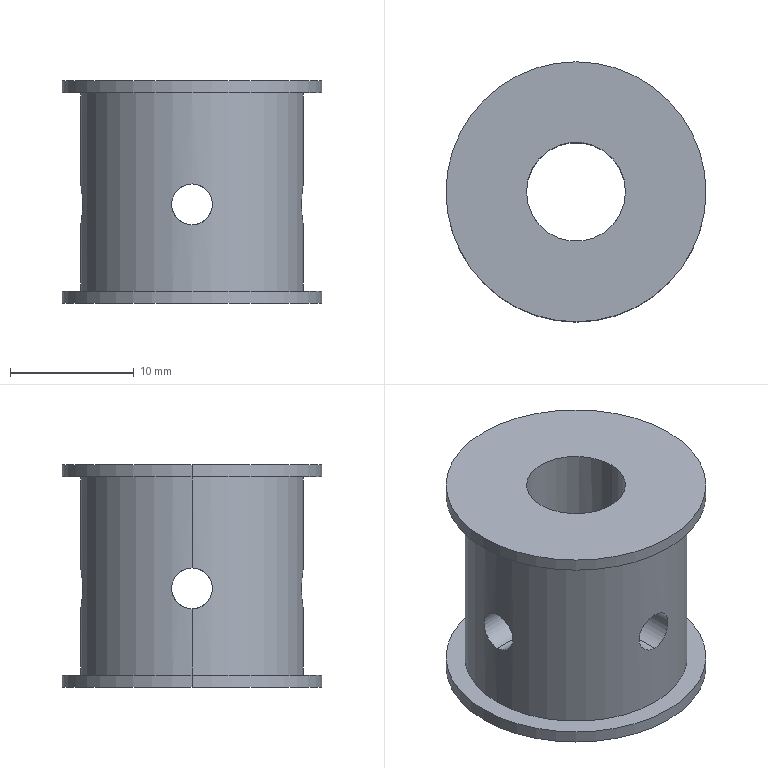Part | STEP file | 11-FG-SZ02211 | 1 solid | 20 faces | box 21 x 21 x 18 mm | volume 3687 mm3 | cylinder 16 | plane 4 | commonest cylinder face diameters 3.3 x8 21 x4 8 x2 18 x2
STEP:
#1=CARTESIAN_POINT('',(0.,-4.,9.65));
#2=VERTEX_POINT('',#1);
#3=CARTESIAN_POINT('',(0.,-4.,6.35));
#4=VERTEX_POINT('',#3);
#5=CARTESIAN_POINT('',(0.,-4.,9.65));
#6=CARTESIAN_POINT('',(0.1103,-4.,9.65));
#7=CARTESIAN_POINT('',(0.2186,-3.995,9.639));
#8=CARTESIAN_POINT('',(0.4313,-3.978,9.596));
#9=CARTESIAN_POINT('',(0.5367,-3.965,9.564));
#10=CARTESIAN_POINT('',(0.8358,-3.917,9.439));
#11=CARTESIAN_POINT('',(1.017,-3.872,9.316));
#12=CARTESIAN_POINT('',(1.318,-3.78,9.015));
#13=CARTESIAN_POINT('',(1.44,-3.733,8.834));
#14=CARTESIAN_POINT('',(1.564,-3.682,8.537));
#15=CARTESIAN_POINT('',(1.596,-3.668,8.432));
#16=CARTESIAN_POINT('',(1.639,-3.649,8.218));
#17=CARTESIAN_POINT('',(1.65,-3.644,8.11));
#18=CARTESIAN_POINT('',(1.65,-3.644,7.892));
#19=CARTESIAN_POINT('',(1.639,-3.649,7.781));
#20=CARTESIAN_POINT('',(1.596,-3.668,7.569));
#21=CARTESIAN_POINT('',(1.565,-3.682,7.465));
#22=CARTESIAN_POINT('',(1.481,-3.716,7.264));
#23=CARTESIAN_POINT('',(1.43,-3.736,7.17));
#24=CARTESIAN_POINT('',(1.311,-3.78,6.992));
#25=CARTESIAN_POINT('',(1.242,-3.803,6.908));
#26=CARTESIAN_POINT('',(1.091,-3.849,6.757));
#27=CARTESIAN_POINT('',(1.009,-3.872,6.69));
#28=CARTESIAN_POINT('',(0.8304,-3.914,6.57));
#29=CARTESIAN_POINT('',(0.7343,-3.933,6.519));
#30=CARTESIAN_POINT('',(0.4369,-3.981,6.394));
#31=CARTESIAN_POINT('',(0.2174,-4.,6.35));
#32=CARTESIAN_POINT('',(0.,-4.,6.35));
#33=B_SPLINE_CURVE_WITH_KNOTS('',3,(#5,#6,#7,#8,#9,#10,#11,#12,#13,#14,#15,#16,#17,#18,#19,#20,#21,#22,#23,#24,#25,#26,#27,#28,#29,#30,#31,#32),.UNSPECIFIED.,.F.,.F.,(4,2,2,2,2,2,2,2,2,2,2,2,2,4),(0.,0.0003261,0.0006522,0.001304,0.001957,0.002283,0.002609,0.002935,0.003261,0.003587,0.003913,0.004239,0.004565,0.005218),.UNSPECIFIED.);
#34=EDGE_CURVE('',#2,#4,#33,.T.);
#35=ORIENTED_EDGE('',*,*,#34,.F.);
#36=CARTESIAN_POINT('',(0.,-4.,6.35));
#37=CARTESIAN_POINT('',(-0.1086,-4.,6.35));
#38=CARTESIAN_POINT('',(-0.2188,-3.995,6.361));
#39=CARTESIAN_POINT('',(-0.4326,-3.978,6.404));
#40=CARTESIAN_POINT('',(-0.5359,-3.965,6.436));
#41=CARTESIAN_POINT('',(-0.8355,-3.917,6.561));
#42=CARTESIAN_POINT('',(-1.016,-3.872,6.682));
#43=CARTESIAN_POINT('',(-1.244,-3.803,6.91));
#44=CARTESIAN_POINT('',(-1.311,-3.78,6.992));
#45=CARTESIAN_POINT('',(-1.43,-3.736,7.17));
#46=CARTESIAN_POINT('',(-1.481,-3.716,7.266));
#47=CARTESIAN_POINT('',(-1.564,-3.682,7.465));
#48=CARTESIAN_POINT('',(-1.596,-3.668,7.567));
#49=CARTESIAN_POINT('',(-1.639,-3.649,7.78));
#50=CARTESIAN_POINT('',(-1.65,-3.644,7.891));
#51=CARTESIAN_POINT('',(-1.65,-3.644,8.217));
#52=CARTESIAN_POINT('',(-1.606,-3.665,8.436));
#53=CARTESIAN_POINT('',(-1.482,-3.716,8.734));
#54=CARTESIAN_POINT('',(-1.43,-3.736,8.83));
#55=CARTESIAN_POINT('',(-1.311,-3.78,9.008));
#56=CARTESIAN_POINT('',(-1.243,-3.803,9.09));
#57=CARTESIAN_POINT('',(-1.092,-3.849,9.242));
#58=CARTESIAN_POINT('',(-1.008,-3.872,9.311));
#59=CARTESIAN_POINT('',(-0.8311,-3.914,9.429));
#60=CARTESIAN_POINT('',(-0.7368,-3.933,9.48));
#61=CARTESIAN_POINT('',(-0.4348,-3.982,9.607));
#62=CARTESIAN_POINT('',(-0.2205,-4.,9.65));
#63=CARTESIAN_POINT('',(0.,-4.,9.65));
#64=B_SPLINE_CURVE_WITH_KNOTS('',3,(#36,#37,#38,#39,#40,#41,#42,#43,#44,#45,#46,#47,#48,#49,#50,#51,#52,#53,#54,#55,#56,#57,#58,#59,#60,#61,#62,#63),.UNSPECIFIED.,.F.,.F.,(4,2,2,2,2,2,2,2,2,2,2,2,2,4),(0.005218,0.005543,0.005869,0.006521,0.006847,0.007173,0.007499,0.007824,0.008476,0.008802,0.009128,0.009454,0.009779,0.01043),.UNSPECIFIED.);
#65=EDGE_CURVE('',#4,#2,#64,.T.);
#66=ORIENTED_EDGE('',*,*,#65,.F.);
#67=EDGE_LOOP('',(#35,#66));
#68=FACE_BOUND('',#67,.T.);
#69=CARTESIAN_POINT('',(4.,0.,18.));
#70=VERTEX_POINT('',#69);
#71=CARTESIAN_POINT('',(-4.,0.,18.));
#72=VERTEX_POINT('',#71);
#73=CARTESIAN_POINT('',(0.,0.,18.));
#74=DIRECTION('',(0.,0.,-1.));
#75=DIRECTION('',(-1.,0.,0.));
#76=AXIS2_PLACEMENT_3D('',#73,#74,#75);
#77=CIRCLE('',#76,4.);
#78=EDGE_CURVE('',#70,#72,#77,.T.);
#79=ORIENTED_EDGE('',*,*,#78,.F.);
#80=CARTESIAN_POINT('',(4.,0.,9.65));
#81=VERTEX_POINT('',#80);
#82=CARTESIAN_POINT('',(4.,0.,18.));
#83=DIRECTION('',(0.,0.,-1.));
#84=VECTOR('',#83,1000.);
#85=LINE('',#82,#84);
#86=EDGE_CURVE('',#70,#81,#85,.T.);
#87=ORIENTED_EDGE('',*,*,#86,.T.);
#88=CARTESIAN_POINT('',(4.,0.,6.35));
#89=VERTEX_POINT('',#88);
#90=CARTESIAN_POINT('',(4.,0.,6.35));
#91=CARTESIAN_POINT('',(4.,-0.1103,6.35));
#92=CARTESIAN_POINT('',(3.995,-0.2186,6.361));
#93=CARTESIAN_POINT('',(3.978,-0.4313,6.404));
#94=CARTESIAN_POINT('',(3.965,-0.5367,6.436));
#95=CARTESIAN_POINT('',(3.917,-0.8358,6.561));
#96=CARTESIAN_POINT('',(3.872,-1.017,6.684));
#97=CARTESIAN_POINT('',(3.78,-1.318,6.985));
#98=CARTESIAN_POINT('',(3.733,-1.44,7.166));
#99=CARTESIAN_POINT('',(3.682,-1.564,7.463));
#100=CARTESIAN_POINT('',(3.668,-1.596,7.568));
#101=CARTESIAN_POINT('',(3.649,-1.639,7.782));
#102=CARTESIAN_POINT('',(3.644,-1.65,7.89));
#103=CARTESIAN_POINT('',(3.644,-1.65,8.108));
#104=CARTESIAN_POINT('',(3.649,-1.639,8.219));
#105=CARTESIAN_POINT('',(3.668,-1.596,8.431));
#106=CARTESIAN_POINT('',(3.682,-1.565,8.535));
#107=CARTESIAN_POINT('',(3.716,-1.481,8.736));
#108=CARTESIAN_POINT('',(3.736,-1.43,8.83));
#109=CARTESIAN_POINT('',(3.78,-1.311,9.008));
#110=CARTESIAN_POINT('',(3.803,-1.242,9.092));
#111=CARTESIAN_POINT('',(3.849,-1.091,9.243));
#112=CARTESIAN_POINT('',(3.872,-1.009,9.31));
#113=CARTESIAN_POINT('',(3.914,-0.8304,9.43));
#114=CARTESIAN_POINT('',(3.933,-0.7343,9.481));
#115=CARTESIAN_POINT('',(3.981,-0.4369,9.606));
#116=CARTESIAN_POINT('',(4.,-0.2174,9.65));
#117=CARTESIAN_POINT('',(4.,0.,9.65));
#118=B_SPLINE_CURVE_WITH_KNOTS('',3,(#90,#91,#92,#93,#94,#95,#96,#97,#98,#99,#100,#101,#102,#103,#104,#105,#106,#107,#108,#109,#110,#111,#112,#113,#114,#115,#116,#117),.UNSPECIFIED.,.F.,.F.,(4,2,2,2,2,2,2,2,2,2,2,2,2,4),(0.,0.0003261,0.0006522,0.001304,0.001957,0.002283,0.002609,0.002935,0.003261,0.003587,0.003913,0.004239,0.004565,0.005218),.UNSPECIFIED.);
#119=EDGE_CURVE('',#89,#81,#118,.T.);
#120=ORIENTED_EDGE('',*,*,#119,.F.);
#121=CARTESIAN_POINT('',(4.,0.,0.));
#122=VERTEX_POINT('',#121);
#123=CARTESIAN_POINT('',(4.,0.,18.));
#124=DIRECTION('',(0.,0.,-1.));
#125=VECTOR('',#124,1000.);
#126=LINE('',#123,#125);
#127=EDGE_CURVE('',#89,#122,#126,.T.);
#128=ORIENTED_EDGE('',*,*,#127,.T.);
#129=CARTESIAN_POINT('',(-4.,0.,0.));
#130=VERTEX_POINT('',#129);
#131=CARTESIAN_POINT('',(0.,0.,0.));
#132=DIRECTION('',(0.,0.,-1.));
#133=DIRECTION('',(-1.,0.,0.));
#134=AXIS2_PLACEMENT_3D('',#131,#132,#133);
#135=CIRCLE('',#134,4.);
#136=EDGE_CURVE('',#122,#130,#135,.T.);
#137=ORIENTED_EDGE('',*,*,#136,.T.);
#138=CARTESIAN_POINT('',(-4.,0.,6.35));
#139=VERTEX_POINT('',#138);
#140=CARTESIAN_POINT('',(-4.,0.,18.));
#141=DIRECTION('',(0.,0.,-1.));
#142=VECTOR('',#141,1000.);
#143=LINE('',#140,#142);
#144=EDGE_CURVE('',#139,#130,#143,.T.);
#145=ORIENTED_EDGE('',*,*,#144,.F.);
#146=CARTESIAN_POINT('',(-4.,0.,9.65));
#147=VERTEX_POINT('',#146);
#148=CARTESIAN_POINT('',(-4.,0.,9.65));
#149=CARTESIAN_POINT('',(-4.,-0.1086,9.65));
#150=CARTESIAN_POINT('',(-3.995,-0.2188,9.639));
#151=CARTESIAN_POINT('',(-3.978,-0.4326,9.596));
#152=CARTESIAN_POINT('',(-3.965,-0.5359,9.564));
#153=CARTESIAN_POINT('',(-3.917,-0.8355,9.439));
#154=CARTESIAN_POINT('',(-3.872,-1.016,9.318));
#155=CARTESIAN_POINT('',(-3.803,-1.244,9.09));
#156=CARTESIAN_POINT('',(-3.78,-1.311,9.008));
#157=CARTESIAN_POINT('',(-3.736,-1.43,8.83));
#158=CARTESIAN_POINT('',(-3.716,-1.481,8.734));
#159=CARTESIAN_POINT('',(-3.682,-1.564,8.535));
#160=CARTESIAN_POINT('',(-3.668,-1.596,8.433));
#161=CARTESIAN_POINT('',(-3.649,-1.639,8.22));
#162=CARTESIAN_POINT('',(-3.644,-1.65,8.109));
#163=CARTESIAN_POINT('',(-3.644,-1.65,7.783));
#164=CARTESIAN_POINT('',(-3.665,-1.606,7.564));
#165=CARTESIAN_POINT('',(-3.716,-1.482,7.266));
#166=CARTESIAN_POINT('',(-3.736,-1.43,7.17));
#167=CARTESIAN_POINT('',(-3.78,-1.311,6.992));
#168=CARTESIAN_POINT('',(-3.803,-1.243,6.91));
#169=CARTESIAN_POINT('',(-3.849,-1.092,6.758));
#170=CARTESIAN_POINT('',(-3.872,-1.008,6.689));
#171=CARTESIAN_POINT('',(-3.914,-0.8311,6.571));
#172=CARTESIAN_POINT('',(-3.933,-0.7368,6.52));
#173=CARTESIAN_POINT('',(-3.982,-0.4348,6.393));
#174=CARTESIAN_POINT('',(-4.,-0.2205,6.35));
#175=CARTESIAN_POINT('',(-4.,0.,6.35));
#176=B_SPLINE_CURVE_WITH_KNOTS('',3,(#148,#149,#150,#151,#152,#153,#154,#155,#156,#157,#158,#159,#160,#161,#162,#163,#164,#165,#166,#167,#168,#169,#170,#171,#172,#173,#174,#175),.UNSPECIFIED.,.F.,.F.,(4,2,2,2,2,2,2,2,2,2,2,2,2,4),(0.005218,0.005543,0.005869,0.006521,0.006847,0.007173,0.007499,0.007824,0.008476,0.008802,0.009128,0.009454,0.009779,0.01043),.UNSPECIFIED.);
#177=EDGE_CURVE('',#147,#139,#176,.T.);
#178=ORIENTED_EDGE('',*,*,#177,.F.);
#179=CARTESIAN_POINT('',(-4.,0.,18.));
#180=DIRECTION('',(0.,0.,-1.));
#181=VECTOR('',#180,1000.);
#182=LINE('',#179,#181);
#183=EDGE_CURVE('',#72,#147,#182,.T.);
#184=ORIENTED_EDGE('',*,*,#183,.F.);
#185=EDGE_LOOP('',(#79,#87,#120,#128,#137,#145,#178,#184));
#186=FACE_OUTER_BOUND('',#185,.T.);
#187=CARTESIAN_POINT('',(0.,0.,18.));
#188=DIRECTION('',(0.,0.,-1.));
#189=DIRECTION('',(-1.,0.,0.));
#190=AXIS2_PLACEMENT_3D('',#187,#188,#189);
#191=CYLINDRICAL_SURFACE('',#190,4.);
#192=ADVANCED_FACE('',(#68,#186),#191,.F.);
#193=CARTESIAN_POINT('',(-9.,0.,9.65));
#194=VERTEX_POINT('',#193);
#195=CARTESIAN_POINT('',(-9.,0.,6.35));
#196=VERTEX_POINT('',#195);
#197=CARTESIAN_POINT('',(-9.,0.,9.65));
#198=CARTESIAN_POINT('',(-9.,-0.1093,9.65));
#199=CARTESIAN_POINT('',(-8.998,-0.2167,9.639));
#200=CARTESIAN_POINT('',(-8.99,-0.4279,9.597));
#201=CARTESIAN_POINT('',(-8.985,-0.5328,9.565));
#202=CARTESIAN_POINT('',(-8.971,-0.7325,9.482));
#203=CARTESIAN_POINT('',(-8.962,-0.8272,9.432));
#204=CARTESIAN_POINT('',(-8.944,-1.006,9.312));
#205=CARTESIAN_POINT('',(-8.934,-1.091,9.242));
#206=CARTESIAN_POINT('',(-8.904,-1.319,9.015));
#207=CARTESIAN_POINT('',(-8.884,-1.442,8.831));
#208=CARTESIAN_POINT('',(-8.856,-1.606,8.434));
#209=CARTESIAN_POINT('',(-8.847,-1.65,8.216));
#210=CARTESIAN_POINT('',(-8.847,-1.65,7.893));
#211=CARTESIAN_POINT('',(-8.849,-1.639,7.783));
#212=CARTESIAN_POINT('',(-8.857,-1.597,7.571));
#213=CARTESIAN_POINT('',(-8.863,-1.566,7.468));
#214=CARTESIAN_POINT('',(-8.884,-1.441,7.168));
#215=CARTESIAN_POINT('',(-8.904,-1.32,6.987));
#216=CARTESIAN_POINT('',(-8.934,-1.09,6.756));
#217=CARTESIAN_POINT('',(-8.944,-1.007,6.688));
#218=CARTESIAN_POINT('',(-8.962,-0.8283,6.569));
#219=CARTESIAN_POINT('',(-8.971,-0.7317,6.517));
#220=CARTESIAN_POINT('',(-8.985,-0.5322,6.434));
#221=CARTESIAN_POINT('',(-8.99,-0.4293,6.403));
#222=CARTESIAN_POINT('',(-8.998,-0.2173,6.361));
#223=CARTESIAN_POINT('',(-9.,-0.1078,6.35));
#224=CARTESIAN_POINT('',(-9.,0.,6.35));
#225=B_SPLINE_CURVE_WITH_KNOTS('',3,(#197,#198,#199,#200,#201,#202,#203,#204,#205,#206,#207,#208,#209,#210,#211,#212,#213,#214,#215,#216,#217,#218,#219,#220,#221,#222,#223,#224),.UNSPECIFIED.,.F.,.F.,(4,2,2,2,2,2,2,2,2,2,2,2,2,4),(0.,0.0003231,0.0006462,0.0009693,0.001292,0.001939,0.002585,0.002908,0.003231,0.003877,0.0042,0.004523,0.004846,0.00517),.UNSPECIFIED.);
#226=EDGE_CURVE('',#194,#196,#225,.T.);
#227=ORIENTED_EDGE('',*,*,#226,.F.);
#228=CARTESIAN_POINT('',(20.,0.,9.65));
#229=DIRECTION('',(1.,0.,0.));
#230=VECTOR('',#229,1000.);
#231=LINE('',#228,#230);
#232=EDGE_CURVE('',#194,#147,#231,.T.);
#233=ORIENTED_EDGE('',*,*,#232,.T.);
#234=ORIENTED_EDGE('',*,*,#177,.T.);
#235=CARTESIAN_POINT('',(20.,0.,6.35));
#236=DIRECTION('',(1.,0.,0.));
#237=VECTOR('',#236,1000.);
#238=LINE('',#235,#237);
#239=EDGE_CURVE('',#196,#139,#238,.T.);
#240=ORIENTED_EDGE('',*,*,#239,.F.);
#241=EDGE_LOOP('',(#227,#233,#234,#240));
#242=FACE_OUTER_BOUND('',#241,.T.);
#243=CARTESIAN_POINT('',(20.,0.,8.));
#244=DIRECTION('',(1.,0.,0.));
#245=DIRECTION('',(0.,0.,-1.));
#246=AXIS2_PLACEMENT_3D('',#243,#244,#245);
#247=CYLINDRICAL_SURFACE('',#246,1.65);
#248=ADVANCED_FACE('',(#242),#247,.F.);
#249=ORIENTED_EDGE('',*,*,#119,.T.);
#250=CARTESIAN_POINT('',(9.,0.,9.65));
#251=VERTEX_POINT('',#250);
#252=CARTESIAN_POINT('',(20.,0.,9.65));
#253=DIRECTION('',(1.,0.,0.));
#254=VECTOR('',#253,1000.);
#255=LINE('',#252,#254);
#256=EDGE_CURVE('',#81,#251,#255,.T.);
#257=ORIENTED_EDGE('',*,*,#256,.T.);
#258=CARTESIAN_POINT('',(9.,0.,6.35));
#259=VERTEX_POINT('',#258);
#260=CARTESIAN_POINT('',(9.,0.,6.35));
#261=CARTESIAN_POINT('',(9.,-0.1093,6.35));
#262=CARTESIAN_POINT('',(8.998,-0.2167,6.361));
#263=CARTESIAN_POINT('',(8.99,-0.4279,6.403));
#264=CARTESIAN_POINT('',(8.985,-0.5328,6.435));
#265=CARTESIAN_POINT('',(8.971,-0.7325,6.518));
#266=CARTESIAN_POINT('',(8.962,-0.8272,6.568));
#267=CARTESIAN_POINT('',(8.944,-1.006,6.688));
#268=CARTESIAN_POINT('',(8.934,-1.091,6.758));
#269=CARTESIAN_POINT('',(8.904,-1.319,6.985));
#270=CARTESIAN_POINT('',(8.884,-1.442,7.169));
#271=CARTESIAN_POINT('',(8.856,-1.606,7.566));
#272=CARTESIAN_POINT('',(8.847,-1.65,7.784));
#273=CARTESIAN_POINT('',(8.847,-1.65,8.107));
#274=CARTESIAN_POINT('',(8.849,-1.639,8.217));
#275=CARTESIAN_POINT('',(8.857,-1.597,8.429));
#276=CARTESIAN_POINT('',(8.863,-1.566,8.532));
#277=CARTESIAN_POINT('',(8.884,-1.441,8.832));
#278=CARTESIAN_POINT('',(8.904,-1.32,9.013));
#279=CARTESIAN_POINT('',(8.934,-1.09,9.244));
#280=CARTESIAN_POINT('',(8.944,-1.007,9.312));
#281=CARTESIAN_POINT('',(8.962,-0.8283,9.431));
#282=CARTESIAN_POINT('',(8.971,-0.7317,9.483));
#283=CARTESIAN_POINT('',(8.985,-0.5322,9.566));
#284=CARTESIAN_POINT('',(8.99,-0.4293,9.597));
#285=CARTESIAN_POINT('',(8.998,-0.2173,9.639));
#286=CARTESIAN_POINT('',(9.,-0.1078,9.65));
#287=CARTESIAN_POINT('',(9.,0.,9.65));
#288=B_SPLINE_CURVE_WITH_KNOTS('',3,(#260,#261,#262,#263,#264,#265,#266,#267,#268,#269,#270,#271,#272,#273,#274,#275,#276,#277,#278,#279,#280,#281,#282,#283,#284,#285,#286,#287),.UNSPECIFIED.,.F.,.F.,(4,2,2,2,2,2,2,2,2,2,2,2,2,4),(0.,0.0003231,0.0006462,0.0009693,0.001292,0.001939,0.002585,0.002908,0.003231,0.003877,0.0042,0.004523,0.004846,0.00517),.UNSPECIFIED.);
#289=EDGE_CURVE('',#259,#251,#288,.T.);
#290=ORIENTED_EDGE('',*,*,#289,.F.);
#291=CARTESIAN_POINT('',(20.,0.,6.35));
#292=DIRECTION('',(1.,0.,0.));
#293=VECTOR('',#292,1000.);
#294=LINE('',#291,#293);
#295=EDGE_CURVE('',#89,#259,#294,.T.);
#296=ORIENTED_EDGE('',*,*,#295,.F.);
#297=EDGE_LOOP('',(#249,#257,#290,#296));
#298=FACE_OUTER_BOUND('',#297,.T.);
#299=CARTESIAN_POINT('',(20.,0.,8.));
#300=DIRECTION('',(1.,0.,0.));
#301=DIRECTION('',(0.,0.,-1.));
#302=AXIS2_PLACEMENT_3D('',#299,#300,#301);
#303=CYLINDRICAL_SURFACE('',#302,1.65);
#304=ADVANCED_FACE('',(#298),#303,.F.);
#305=CARTESIAN_POINT('',(0.,-9.,6.35));
#306=VERTEX_POINT('',#305);
#307=CARTESIAN_POINT('',(0.,-9.,9.65));
#308=VERTEX_POINT('',#307);
#309=CARTESIAN_POINT('',(0.,-9.,6.35));
#310=CARTESIAN_POINT('',(-0.2156,-9.,6.35));
#311=CARTESIAN_POINT('',(-0.4331,-8.992,6.393));
#312=CARTESIAN_POINT('',(-0.8303,-8.964,6.558));
#313=CARTESIAN_POINT('',(-1.014,-8.944,6.681));
#314=CARTESIAN_POINT('',(-1.242,-8.914,6.909));
#315=CARTESIAN_POINT('',(-1.312,-8.904,6.993));
#316=CARTESIAN_POINT('',(-1.431,-8.886,7.172));
#317=CARTESIAN_POINT('',(-1.482,-8.877,7.267));
#318=CARTESIAN_POINT('',(-1.607,-8.856,7.567));
#319=CARTESIAN_POINT('',(-1.65,-8.847,7.781));
#320=CARTESIAN_POINT('',(-1.65,-8.847,8.108));
#321=CARTESIAN_POINT('',(-1.639,-8.849,8.215));
#322=CARTESIAN_POINT('',(-1.598,-8.857,8.427));
#323=CARTESIAN_POINT('',(-1.566,-8.863,8.532));
#324=CARTESIAN_POINT('',(-1.483,-8.877,8.731));
#325=CARTESIAN_POINT('',(-1.432,-8.885,8.826));
#326=CARTESIAN_POINT('',(-1.313,-8.904,9.006));
#327=CARTESIAN_POINT('',(-1.243,-8.914,9.09));
#328=CARTESIAN_POINT('',(-1.016,-8.944,9.318));
#329=CARTESIAN_POINT('',(-0.8322,-8.964,9.441));
#330=CARTESIAN_POINT('',(-0.4354,-8.992,9.606));
#331=CARTESIAN_POINT('',(-0.2185,-9.,9.65));
#332=CARTESIAN_POINT('',(0.,-9.,9.65));
#333=B_SPLINE_CURVE_WITH_KNOTS('',3,(#309,#310,#311,#312,#313,#314,#315,#316,#317,#318,#319,#320,#321,#322,#323,#324,#325,#326,#327,#328,#329,#330,#331,#332),.UNSPECIFIED.,.F.,.F.,(4,2,2,2,2,2,2,2,2,2,2,4),(0.00517,0.005816,0.006462,0.006785,0.007108,0.007754,0.008077,0.0084,0.008723,0.009046,0.009692,0.01034),.UNSPECIFIED.);
#334=EDGE_CURVE('',#306,#308,#333,.T.);
#335=ORIENTED_EDGE('',*,*,#334,.F.);
#336=CARTESIAN_POINT('',(0.,20.,6.35));
#337=DIRECTION('',(0.,1.,0.));
#338=VECTOR('',#337,1000.);
#339=LINE('',#336,#338);
#340=EDGE_CURVE('',#306,#4,#339,.T.);
#341=ORIENTED_EDGE('',*,*,#340,.T.);
#342=ORIENTED_EDGE('',*,*,#65,.T.);
#343=CARTESIAN_POINT('',(0.,20.,9.65));
#344=DIRECTION('',(0.,1.,0.));
#345=VECTOR('',#344,1000.);
#346=LINE('',#343,#345);
#347=EDGE_CURVE('',#308,#2,#346,.T.);
#348=ORIENTED_EDGE('',*,*,#347,.F.);
#349=EDGE_LOOP('',(#335,#341,#342,#348));
#350=FACE_OUTER_BOUND('',#349,.T.);
#351=CARTESIAN_POINT('',(0.,20.,8.));
#352=DIRECTION('',(0.,1.,0.));
#353=DIRECTION('',(0.,0.,1.));
#354=AXIS2_PLACEMENT_3D('',#351,#352,#353);
#355=CYLINDRICAL_SURFACE('',#354,1.65);
#356=ADVANCED_FACE('',(#350),#355,.F.);
#357=CARTESIAN_POINT('',(10.5,0.,18.));
#358=VERTEX_POINT('',#357);
#359=CARTESIAN_POINT('',(-10.5,0.,18.));
#360=VERTEX_POINT('',#359);
#361=CARTESIAN_POINT('',(0.,0.,18.));
#362=DIRECTION('',(0.,0.,1.));
#363=DIRECTION('',(1.,0.,0.));
#364=AXIS2_PLACEMENT_3D('',#361,#362,#363);
#365=CIRCLE('',#364,10.5);
#366=EDGE_CURVE('',#358,#360,#365,.T.);
#367=ORIENTED_EDGE('',*,*,#366,.F.);
#368=CARTESIAN_POINT('',(10.5,0.,17.));
#369=VERTEX_POINT('',#368);
#370=CARTESIAN_POINT('',(10.5,0.,18.));
#371=DIRECTION('',(0.,0.,-1.));
#372=VECTOR('',#371,1000.);
#373=LINE('',#370,#372);
#374=EDGE_CURVE('',#358,#369,#373,.T.);
#375=ORIENTED_EDGE('',*,*,#374,.T.);
#376=CARTESIAN_POINT('',(-10.5,0.,17.));
#377=VERTEX_POINT('',#376);
#378=CARTESIAN_POINT('',(0.,0.,17.));
#379=DIRECTION('',(0.,0.,1.));
#380=DIRECTION('',(1.,0.,0.));
#381=AXIS2_PLACEMENT_3D('',#378,#379,#380);
#382=CIRCLE('',#381,10.5);
#383=EDGE_CURVE('',#369,#377,#382,.T.);
#384=ORIENTED_EDGE('',*,*,#383,.T.);
#385=CARTESIAN_POINT('',(-10.5,0.,18.));
#386=DIRECTION('',(0.,0.,-1.));
#387=VECTOR('',#386,1000.);
#388=LINE('',#385,#387);
#389=EDGE_CURVE('',#360,#377,#388,.T.);
#390=ORIENTED_EDGE('',*,*,#389,.F.);
#391=EDGE_LOOP('',(#367,#375,#384,#390));
#392=FACE_OUTER_BOUND('',#391,.T.);
#393=CARTESIAN_POINT('',(0.,0.,18.));
#394=DIRECTION('',(0.,0.,-1.));
#395=DIRECTION('',(-1.,0.,0.));
#396=AXIS2_PLACEMENT_3D('',#393,#394,#395);
#397=CYLINDRICAL_SURFACE('',#396,10.5);
#398=ADVANCED_FACE('',(#392),#397,.T.);
#399=CARTESIAN_POINT('',(0.,9.,9.65));
#400=VERTEX_POINT('',#399);
#401=CARTESIAN_POINT('',(0.,9.,6.35));
#402=VERTEX_POINT('',#401);
#403=CARTESIAN_POINT('',(0.,9.,9.65));
#404=CARTESIAN_POINT('',(-0.1093,9.,9.65));
#405=CARTESIAN_POINT('',(-0.2167,8.998,9.639));
#406=CARTESIAN_POINT('',(-0.4279,8.99,9.597));
#407=CARTESIAN_POINT('',(-0.5328,8.985,9.565));
#408=CARTESIAN_POINT('',(-0.7325,8.971,9.482));
#409=CARTESIAN_POINT('',(-0.8272,8.962,9.432));
#410=CARTESIAN_POINT('',(-1.006,8.944,9.312));
#411=CARTESIAN_POINT('',(-1.091,8.934,9.242));
#412=CARTESIAN_POINT('',(-1.319,8.904,9.015));
#413=CARTESIAN_POINT('',(-1.442,8.884,8.831));
#414=CARTESIAN_POINT('',(-1.606,8.856,8.434));
#415=CARTESIAN_POINT('',(-1.65,8.847,8.216));
#416=CARTESIAN_POINT('',(-1.65,8.847,7.893));
#417=CARTESIAN_POINT('',(-1.639,8.849,7.783));
#418=CARTESIAN_POINT('',(-1.597,8.857,7.571));
#419=CARTESIAN_POINT('',(-1.566,8.863,7.468));
#420=CARTESIAN_POINT('',(-1.441,8.884,7.168));
#421=CARTESIAN_POINT('',(-1.32,8.904,6.987));
#422=CARTESIAN_POINT('',(-1.09,8.934,6.756));
#423=CARTESIAN_POINT('',(-1.007,8.944,6.688));
#424=CARTESIAN_POINT('',(-0.8283,8.962,6.569));
#425=CARTESIAN_POINT('',(-0.7317,8.971,6.517));
#426=CARTESIAN_POINT('',(-0.5322,8.985,6.434));
#427=CARTESIAN_POINT('',(-0.4293,8.99,6.403));
#428=CARTESIAN_POINT('',(-0.2173,8.998,6.361));
#429=CARTESIAN_POINT('',(-0.1078,9.,6.35));
#430=CARTESIAN_POINT('',(0.,9.,6.35));
#431=B_SPLINE_CURVE_WITH_KNOTS('',3,(#403,#404,#405,#406,#407,#408,#409,#410,#411,#412,#413,#414,#415,#416,#417,#418,#419,#420,#421,#422,#423,#424,#425,#426,#427,#428,#429,#430),.UNSPECIFIED.,.F.,.F.,(4,2,2,2,2,2,2,2,2,2,2,2,2,4),(0.,0.0003231,0.0006462,0.0009693,0.001292,0.001939,0.002585,0.002908,0.003231,0.003877,0.0042,0.004523,0.004846,0.00517),.UNSPECIFIED.);
#432=EDGE_CURVE('',#400,#402,#431,.T.);
#433=ORIENTED_EDGE('',*,*,#432,.T.);
#434=CARTESIAN_POINT('',(0.,9.,6.35));
#435=CARTESIAN_POINT('',(0.2156,9.,6.35));
#436=CARTESIAN_POINT('',(0.4331,8.992,6.393));
#437=CARTESIAN_POINT('',(0.8303,8.964,6.558));
#438=CARTESIAN_POINT('',(1.014,8.944,6.681));
#439=CARTESIAN_POINT('',(1.242,8.914,6.909));
#440=CARTESIAN_POINT('',(1.312,8.904,6.993));
#441=CARTESIAN_POINT('',(1.431,8.886,7.172));
#442=CARTESIAN_POINT('',(1.482,8.877,7.267));
#443=CARTESIAN_POINT('',(1.607,8.856,7.567));
#444=CARTESIAN_POINT('',(1.65,8.847,7.781));
#445=CARTESIAN_POINT('',(1.65,8.847,8.108));
#446=CARTESIAN_POINT('',(1.639,8.849,8.215));
#447=CARTESIAN_POINT('',(1.598,8.857,8.427));
#448=CARTESIAN_POINT('',(1.566,8.863,8.532));
#449=CARTESIAN_POINT('',(1.483,8.877,8.731));
#450=CARTESIAN_POINT('',(1.432,8.885,8.826));
#451=CARTESIAN_POINT('',(1.313,8.904,9.006));
#452=CARTESIAN_POINT('',(1.243,8.914,9.09));
#453=CARTESIAN_POINT('',(1.016,8.944,9.318));
#454=CARTESIAN_POINT('',(0.8322,8.964,9.441));
#455=CARTESIAN_POINT('',(0.4354,8.992,9.606));
#456=CARTESIAN_POINT('',(0.2185,9.,9.65));
#457=CARTESIAN_POINT('',(0.,9.,9.65));
#458=B_SPLINE_CURVE_WITH_KNOTS('',3,(#434,#435,#436,#437,#438,#439,#440,#441,#442,#443,#444,#445,#446,#447,#448,#449,#450,#451,#452,#453,#454,#455,#456,#457),.UNSPECIFIED.,.F.,.F.,(4,2,2,2,2,2,2,2,2,2,2,4),(0.00517,0.005816,0.006462,0.006785,0.007108,0.007754,0.008077,0.0084,0.008723,0.009046,0.009692,0.01034),.UNSPECIFIED.);
#459=EDGE_CURVE('',#402,#400,#458,.T.);
#460=ORIENTED_EDGE('',*,*,#459,.T.);
#461=EDGE_LOOP('',(#433,#460));
#462=FACE_BOUND('',#461,.T.);
#463=CARTESIAN_POINT('',(9.,0.,17.));
#464=VERTEX_POINT('',#463);
#465=CARTESIAN_POINT('',(-9.,0.,17.));
#466=VERTEX_POINT('',#465);
#467=CARTESIAN_POINT('',(0.,0.,17.));
#468=DIRECTION('',(0.,0.,1.));
#469=DIRECTION('',(1.,0.,0.));
#470=AXIS2_PLACEMENT_3D('',#467,#468,#469);
#471=CIRCLE('',#470,9.);
#472=EDGE_CURVE('',#464,#466,#471,.T.);
#473=ORIENTED_EDGE('',*,*,#472,.F.);
#474=CARTESIAN_POINT('',(9.,0.,17.));
#475=DIRECTION('',(0.,0.,-1.));
#476=VECTOR('',#475,1000.);
#477=LINE('',#474,#476);
#478=EDGE_CURVE('',#464,#251,#477,.T.);
#479=ORIENTED_EDGE('',*,*,#478,.T.);
#480=CARTESIAN_POINT('',(9.,0.,9.65));
#481=CARTESIAN_POINT('',(9.,0.2156,9.65));
#482=CARTESIAN_POINT('',(8.992,0.4331,9.607));
#483=CARTESIAN_POINT('',(8.964,0.8303,9.442));
#484=CARTESIAN_POINT('',(8.944,1.014,9.319));
#485=CARTESIAN_POINT('',(8.914,1.242,9.091));
#486=CARTESIAN_POINT('',(8.904,1.312,9.007));
#487=CARTESIAN_POINT('',(8.886,1.431,8.828));
#488=CARTESIAN_POINT('',(8.877,1.482,8.733));
#489=CARTESIAN_POINT('',(8.856,1.607,8.433));
#490=CARTESIAN_POINT('',(8.847,1.65,8.219));
#491=CARTESIAN_POINT('',(8.847,1.65,7.892));
#492=CARTESIAN_POINT('',(8.849,1.639,7.785));
#493=CARTESIAN_POINT('',(8.857,1.598,7.573));
#494=CARTESIAN_POINT('',(8.863,1.566,7.468));
#495=CARTESIAN_POINT('',(8.877,1.483,7.269));
#496=CARTESIAN_POINT('',(8.885,1.432,7.174));
#497=CARTESIAN_POINT('',(8.904,1.313,6.994));
#498=CARTESIAN_POINT('',(8.914,1.243,6.91));
#499=CARTESIAN_POINT('',(8.944,1.016,6.682));
#500=CARTESIAN_POINT('',(8.964,0.8322,6.559));
#501=CARTESIAN_POINT('',(8.992,0.4354,6.394));
#502=CARTESIAN_POINT('',(9.,0.2185,6.35));
#503=CARTESIAN_POINT('',(9.,0.,6.35));
#504=B_SPLINE_CURVE_WITH_KNOTS('',3,(#480,#481,#482,#483,#484,#485,#486,#487,#488,#489,#490,#491,#492,#493,#494,#495,#496,#497,#498,#499,#500,#501,#502,#503),.UNSPECIFIED.,.F.,.F.,(4,2,2,2,2,2,2,2,2,2,2,4),(0.00517,0.005816,0.006462,0.006785,0.007108,0.007754,0.008077,0.0084,0.008723,0.009046,0.009692,0.01034),.UNSPECIFIED.);
#505=EDGE_CURVE('',#251,#259,#504,.T.);
#506=ORIENTED_EDGE('',*,*,#505,.T.);
#507=CARTESIAN_POINT('',(9.,0.,1.));
#508=VERTEX_POINT('',#507);
#509=CARTESIAN_POINT('',(9.,0.,17.));
#510=DIRECTION('',(0.,0.,-1.));
#511=VECTOR('',#510,1000.);
#512=LINE('',#509,#511);
#513=EDGE_CURVE('',#259,#508,#512,.T.);
#514=ORIENTED_EDGE('',*,*,#513,.T.);
#515=CARTESIAN_POINT('',(-9.,0.,1.));
#516=VERTEX_POINT('',#515);
#517=CARTESIAN_POINT('',(0.,0.,1.));
#518=DIRECTION('',(0.,0.,1.));
#519=DIRECTION('',(1.,0.,0.));
#520=AXIS2_PLACEMENT_3D('',#517,#518,#519);
#521=CIRCLE('',#520,9.);
#522=EDGE_CURVE('',#508,#516,#521,.T.);
#523=ORIENTED_EDGE('',*,*,#522,.T.);
#524=CARTESIAN_POINT('',(-9.,0.,17.));
#525=DIRECTION('',(0.,0.,-1.));
#526=VECTOR('',#525,1000.);
#527=LINE('',#524,#526);
#528=EDGE_CURVE('',#196,#516,#527,.T.);
#529=ORIENTED_EDGE('',*,*,#528,.F.);
#530=CARTESIAN_POINT('',(-9.,0.,6.35));
#531=CARTESIAN_POINT('',(-9.,0.2156,6.35));
#532=CARTESIAN_POINT('',(-8.992,0.4331,6.393));
#533=CARTESIAN_POINT('',(-8.964,0.8303,6.558));
#534=CARTESIAN_POINT('',(-8.944,1.014,6.681));
#535=CARTESIAN_POINT('',(-8.914,1.242,6.909));
#536=CARTESIAN_POINT('',(-8.904,1.312,6.993));
#537=CARTESIAN_POINT('',(-8.886,1.431,7.172));
#538=CARTESIAN_POINT('',(-8.877,1.482,7.267));
#539=CARTESIAN_POINT('',(-8.856,1.607,7.567));
#540=CARTESIAN_POINT('',(-8.847,1.65,7.781));
#541=CARTESIAN_POINT('',(-8.847,1.65,8.108));
#542=CARTESIAN_POINT('',(-8.849,1.639,8.215));
#543=CARTESIAN_POINT('',(-8.857,1.598,8.427));
#544=CARTESIAN_POINT('',(-8.863,1.566,8.532));
#545=CARTESIAN_POINT('',(-8.877,1.483,8.731));
#546=CARTESIAN_POINT('',(-8.885,1.432,8.826));
#547=CARTESIAN_POINT('',(-8.904,1.313,9.006));
#548=CARTESIAN_POINT('',(-8.914,1.243,9.09));
#549=CARTESIAN_POINT('',(-8.944,1.016,9.318));
#550=CARTESIAN_POINT('',(-8.964,0.8322,9.441));
#551=CARTESIAN_POINT('',(-8.992,0.4354,9.606));
#552=CARTESIAN_POINT('',(-9.,0.2185,9.65));
#553=CARTESIAN_POINT('',(-9.,0.,9.65));
#554=B_SPLINE_CURVE_WITH_KNOTS('',3,(#530,#531,#532,#533,#534,#535,#536,#537,#538,#539,#540,#541,#542,#543,#544,#545,#546,#547,#548,#549,#550,#551,#552,#553),.UNSPECIFIED.,.F.,.F.,(4,2,2,2,2,2,2,2,2,2,2,4),(0.00517,0.005816,0.006462,0.006785,0.007108,0.007754,0.008077,0.0084,0.008723,0.009046,0.009692,0.01034),.UNSPECIFIED.);
#555=EDGE_CURVE('',#196,#194,#554,.T.);
#556=ORIENTED_EDGE('',*,*,#555,.T.);
#557=CARTESIAN_POINT('',(-9.,0.,17.));
#558=DIRECTION('',(0.,0.,-1.));
#559=VECTOR('',#558,1000.);
#560=LINE('',#557,#559);
#561=EDGE_CURVE('',#466,#194,#560,.T.);
#562=ORIENTED_EDGE('',*,*,#561,.F.);
#563=EDGE_LOOP('',(#473,#479,#506,#514,#523,#529,#556,#562));
#564=FACE_OUTER_BOUND('',#563,.T.);
#565=CARTESIAN_POINT('',(0.,0.,17.));
#566=DIRECTION('',(0.,0.,-1.));
#567=DIRECTION('',(-1.,0.,0.));
#568=AXIS2_PLACEMENT_3D('',#565,#566,#567);
#569=CYLINDRICAL_SURFACE('',#568,9.);
#570=ADVANCED_FACE('',(#462,#564),#569,.T.);
#571=CARTESIAN_POINT('',(10.5,0.,1.));
#572=VERTEX_POINT('',#571);
#573=CARTESIAN_POINT('',(-10.5,0.,1.));
#574=VERTEX_POINT('',#573);
#575=CARTESIAN_POINT('',(0.,0.,1.));
#576=DIRECTION('',(0.,0.,1.));
#577=DIRECTION('',(1.,0.,0.));
#578=AXIS2_PLACEMENT_3D('',#575,#576,#577);
#579=CIRCLE('',#578,10.5);
#580=EDGE_CURVE('',#572,#574,#579,.T.);
#581=ORIENTED_EDGE('',*,*,#580,.F.);
#582=CARTESIAN_POINT('',(10.5,0.,0.));
#583=VERTEX_POINT('',#582);
#584=CARTESIAN_POINT('',(10.5,0.,1.));
#585=DIRECTION('',(0.,0.,-1.));
#586=VECTOR('',#585,1000.);
#587=LINE('',#584,#586);
#588=EDGE_CURVE('',#572,#583,#587,.T.);
#589=ORIENTED_EDGE('',*,*,#588,.T.);
#590=CARTESIAN_POINT('',(-10.5,0.,0.));
#591=VERTEX_POINT('',#590);
#592=CARTESIAN_POINT('',(0.,0.,0.));
#593=DIRECTION('',(0.,0.,1.));
#594=DIRECTION('',(1.,0.,0.));
#595=AXIS2_PLACEMENT_3D('',#592,#593,#594);
#596=CIRCLE('',#595,10.5);
#597=EDGE_CURVE('',#583,#591,#596,.T.);
#598=ORIENTED_EDGE('',*,*,#597,.T.);
#599=CARTESIAN_POINT('',(-10.5,0.,1.));
#600=DIRECTION('',(0.,0.,-1.));
#601=VECTOR('',#600,1000.);
#602=LINE('',#599,#601);
#603=EDGE_CURVE('',#574,#591,#602,.T.);
#604=ORIENTED_EDGE('',*,*,#603,.F.);
#605=EDGE_LOOP('',(#581,#589,#598,#604));
#606=FACE_OUTER_BOUND('',#605,.T.);
#607=CARTESIAN_POINT('',(0.,0.,1.));
#608=DIRECTION('',(0.,0.,-1.));
#609=DIRECTION('',(-1.,0.,0.));
#610=AXIS2_PLACEMENT_3D('',#607,#608,#609);
#611=CYLINDRICAL_SURFACE('',#610,10.5);
#612=ADVANCED_FACE('',(#606),#611,.T.);
#613=CARTESIAN_POINT('',(0.,4.,9.65));
#614=VERTEX_POINT('',#613);
#615=CARTESIAN_POINT('',(0.,4.,6.35));
#616=VERTEX_POINT('',#615);
#617=CARTESIAN_POINT('',(0.,4.,9.65));
#618=CARTESIAN_POINT('',(-0.1103,4.,9.65));
#619=CARTESIAN_POINT('',(-0.2186,3.995,9.639));
#620=CARTESIAN_POINT('',(-0.4313,3.978,9.596));
#621=CARTESIAN_POINT('',(-0.5367,3.965,9.564));
#622=CARTESIAN_POINT('',(-0.8358,3.917,9.439));
#623=CARTESIAN_POINT('',(-1.017,3.872,9.316));
#624=CARTESIAN_POINT('',(-1.318,3.78,9.015));
#625=CARTESIAN_POINT('',(-1.44,3.733,8.834));
#626=CARTESIAN_POINT('',(-1.564,3.682,8.537));
#627=CARTESIAN_POINT('',(-1.596,3.668,8.432));
#628=CARTESIAN_POINT('',(-1.639,3.649,8.218));
#629=CARTESIAN_POINT('',(-1.65,3.644,8.11));
#630=CARTESIAN_POINT('',(-1.65,3.644,7.892));
#631=CARTESIAN_POINT('',(-1.639,3.649,7.781));
#632=CARTESIAN_POINT('',(-1.596,3.668,7.569));
#633=CARTESIAN_POINT('',(-1.565,3.682,7.465));
#634=CARTESIAN_POINT('',(-1.481,3.716,7.264));
#635=CARTESIAN_POINT('',(-1.43,3.736,7.17));
#636=CARTESIAN_POINT('',(-1.311,3.78,6.992));
#637=CARTESIAN_POINT('',(-1.242,3.803,6.908));
#638=CARTESIAN_POINT('',(-1.091,3.849,6.757));
#639=CARTESIAN_POINT('',(-1.009,3.872,6.69));
#640=CARTESIAN_POINT('',(-0.8304,3.914,6.57));
#641=CARTESIAN_POINT('',(-0.7343,3.933,6.519));
#642=CARTESIAN_POINT('',(-0.4369,3.981,6.394));
#643=CARTESIAN_POINT('',(-0.2174,4.,6.35));
#644=CARTESIAN_POINT('',(0.,4.,6.35));
#645=B_SPLINE_CURVE_WITH_KNOTS('',3,(#617,#618,#619,#620,#621,#622,#623,#624,#625,#626,#627,#628,#629,#630,#631,#632,#633,#634,#635,#636,#637,#638,#639,#640,#641,#642,#643,#644),.UNSPECIFIED.,.F.,.F.,(4,2,2,2,2,2,2,2,2,2,2,2,2,4),(0.,0.0003261,0.0006522,0.001304,0.001957,0.002283,0.002609,0.002935,0.003261,0.003587,0.003913,0.004239,0.004565,0.005218),.UNSPECIFIED.);
#646=EDGE_CURVE('',#614,#616,#645,.T.);
#647=ORIENTED_EDGE('',*,*,#646,.T.);
#648=CARTESIAN_POINT('',(0.,20.,6.35));
#649=DIRECTION('',(0.,1.,0.));
#650=VECTOR('',#649,1000.);
#651=LINE('',#648,#650);
#652=EDGE_CURVE('',#616,#402,#651,.T.);
#653=ORIENTED_EDGE('',*,*,#652,.T.);
#654=ORIENTED_EDGE('',*,*,#432,.F.);
#655=CARTESIAN_POINT('',(0.,20.,9.65));
#656=DIRECTION('',(0.,1.,0.));
#657=VECTOR('',#656,1000.);
#658=LINE('',#655,#657);
#659=EDGE_CURVE('',#614,#400,#658,.T.);
#660=ORIENTED_EDGE('',*,*,#659,.F.);
#661=EDGE_LOOP('',(#647,#653,#654,#660));
#662=FACE_OUTER_BOUND('',#661,.T.);
#663=CARTESIAN_POINT('',(0.,20.,8.));
#664=DIRECTION('',(0.,1.,0.));
#665=DIRECTION('',(0.,0.,1.));
#666=AXIS2_PLACEMENT_3D('',#663,#664,#665);
#667=CYLINDRICAL_SURFACE('',#666,1.65);
#668=ADVANCED_FACE('',(#662),#667,.F.);
#669=ORIENTED_EDGE('',*,*,#652,.F.);
#670=CARTESIAN_POINT('',(0.,4.,6.35));
#671=CARTESIAN_POINT('',(0.1086,4.,6.35));
#672=CARTESIAN_POINT('',(0.2188,3.995,6.361));
#673=CARTESIAN_POINT('',(0.4326,3.978,6.404));
#674=CARTESIAN_POINT('',(0.5359,3.965,6.436));
#675=CARTESIAN_POINT('',(0.8355,3.917,6.561));
#676=CARTESIAN_POINT('',(1.016,3.872,6.682));
#677=CARTESIAN_POINT('',(1.244,3.803,6.91));
#678=CARTESIAN_POINT('',(1.311,3.78,6.992));
#679=CARTESIAN_POINT('',(1.43,3.736,7.17));
#680=CARTESIAN_POINT('',(1.481,3.716,7.266));
#681=CARTESIAN_POINT('',(1.564,3.682,7.465));
#682=CARTESIAN_POINT('',(1.596,3.668,7.567));
#683=CARTESIAN_POINT('',(1.639,3.649,7.78));
#684=CARTESIAN_POINT('',(1.65,3.644,7.891));
#685=CARTESIAN_POINT('',(1.65,3.644,8.217));
#686=CARTESIAN_POINT('',(1.606,3.665,8.436));
#687=CARTESIAN_POINT('',(1.482,3.716,8.734));
#688=CARTESIAN_POINT('',(1.43,3.736,8.83));
#689=CARTESIAN_POINT('',(1.311,3.78,9.008));
#690=CARTESIAN_POINT('',(1.243,3.803,9.09));
#691=CARTESIAN_POINT('',(1.092,3.849,9.242));
#692=CARTESIAN_POINT('',(1.008,3.872,9.311));
#693=CARTESIAN_POINT('',(0.8311,3.914,9.429));
#694=CARTESIAN_POINT('',(0.7368,3.933,9.48));
#695=CARTESIAN_POINT('',(0.4348,3.982,9.607));
#696=CARTESIAN_POINT('',(0.2205,4.,9.65));
#697=CARTESIAN_POINT('',(0.,4.,9.65));
#698=B_SPLINE_CURVE_WITH_KNOTS('',3,(#670,#671,#672,#673,#674,#675,#676,#677,#678,#679,#680,#681,#682,#683,#684,#685,#686,#687,#688,#689,#690,#691,#692,#693,#694,#695,#696,#697),.UNSPECIFIED.,.F.,.F.,(4,2,2,2,2,2,2,2,2,2,2,2,2,4),(0.005218,0.005543,0.005869,0.006521,0.006847,0.007173,0.007499,0.007824,0.008476,0.008802,0.009128,0.009454,0.009779,0.01043),.UNSPECIFIED.);
#699=EDGE_CURVE('',#616,#614,#698,.T.);
#700=ORIENTED_EDGE('',*,*,#699,.T.);
#701=ORIENTED_EDGE('',*,*,#659,.T.);
#702=ORIENTED_EDGE('',*,*,#459,.F.);
#703=EDGE_LOOP('',(#669,#700,#701,#702));
#704=FACE_OUTER_BOUND('',#703,.T.);
#705=CARTESIAN_POINT('',(0.,20.,8.));
#706=DIRECTION('',(0.,1.,0.));
#707=DIRECTION('',(0.,0.,1.));
#708=AXIS2_PLACEMENT_3D('',#705,#706,#707);
#709=CYLINDRICAL_SURFACE('',#708,1.65);
#710=ADVANCED_FACE('',(#704),#709,.F.);
#711=ORIENTED_EDGE('',*,*,#588,.F.);
#712=CARTESIAN_POINT('',(0.,0.,1.));
#713=DIRECTION('',(0.,0.,1.));
#714=DIRECTION('',(1.,0.,0.));
#715=AXIS2_PLACEMENT_3D('',#712,#713,#714);
#716=CIRCLE('',#715,10.5);
#717=EDGE_CURVE('',#574,#572,#716,.T.);
#718=ORIENTED_EDGE('',*,*,#717,.F.);
#719=ORIENTED_EDGE('',*,*,#603,.T.);
#720=CARTESIAN_POINT('',(0.,0.,0.));
#721=DIRECTION('',(0.,0.,1.));
#722=DIRECTION('',(1.,0.,0.));
#723=AXIS2_PLACEMENT_3D('',#720,#721,#722);
#724=CIRCLE('',#723,10.5);
#725=EDGE_CURVE('',#591,#583,#724,.T.);
#726=ORIENTED_EDGE('',*,*,#725,.T.);
#727=EDGE_LOOP('',(#711,#718,#719,#726));
#728=FACE_OUTER_BOUND('',#727,.T.);
#729=CARTESIAN_POINT('',(0.,0.,1.));
#730=DIRECTION('',(0.,0.,-1.));
#731=DIRECTION('',(-1.,0.,0.));
#732=AXIS2_PLACEMENT_3D('',#729,#730,#731);
#733=CYLINDRICAL_SURFACE('',#732,10.5);
#734=ADVANCED_FACE('',(#728),#733,.T.);
#735=CARTESIAN_POINT('',(0.,0.,1.));
#736=DIRECTION('',(0.,0.,1.));
#737=DIRECTION('',(1.,0.,0.));
#738=AXIS2_PLACEMENT_3D('',#735,#736,#737);
#739=CIRCLE('',#738,9.);
#740=EDGE_CURVE('',#516,#508,#739,.T.);
#741=ORIENTED_EDGE('',*,*,#740,.F.);
#742=ORIENTED_EDGE('',*,*,#522,.F.);
#743=EDGE_LOOP('',(#741,#742));
#744=FACE_BOUND('',#743,.T.);
#745=ORIENTED_EDGE('',*,*,#717,.T.);
#746=ORIENTED_EDGE('',*,*,#580,.T.);
#747=EDGE_LOOP('',(#745,#746));
#748=FACE_OUTER_BOUND('',#747,.T.);
#749=CARTESIAN_POINT('',(0.,0.,1.));
#750=DIRECTION('',(0.,0.,1.));
#751=DIRECTION('',(1.,0.,0.));
#752=AXIS2_PLACEMENT_3D('',#749,#750,#751);
#753=PLANE('',#752);
#754=ADVANCED_FACE('',(#744,#748),#753,.T.);
#755=CARTESIAN_POINT('',(0.,0.,0.));
#756=DIRECTION('',(0.,0.,-1.));
#757=DIRECTION('',(-1.,0.,0.));
#758=AXIS2_PLACEMENT_3D('',#755,#756,#757);
#759=CIRCLE('',#758,4.);
#760=EDGE_CURVE('',#130,#122,#759,.T.);
#761=ORIENTED_EDGE('',*,*,#760,.F.);
#762=ORIENTED_EDGE('',*,*,#136,.F.);
#763=EDGE_LOOP('',(#761,#762));
#764=FACE_BOUND('',#763,.T.);
#765=ORIENTED_EDGE('',*,*,#725,.F.);
#766=ORIENTED_EDGE('',*,*,#597,.F.);
#767=EDGE_LOOP('',(#765,#766));
#768=FACE_OUTER_BOUND('',#767,.T.);
#769=CARTESIAN_POINT('',(0.,0.,0.));
#770=DIRECTION('',(0.,0.,1.));
#771=DIRECTION('',(1.,0.,0.));
#772=AXIS2_PLACEMENT_3D('',#769,#770,#771);
#773=PLANE('',#772);
#774=ADVANCED_FACE('',(#764,#768),#773,.F.);
#775=ORIENTED_EDGE('',*,*,#478,.F.);
#776=CARTESIAN_POINT('',(0.,0.,17.));
#777=DIRECTION('',(0.,0.,1.));
#778=DIRECTION('',(1.,0.,0.));
#779=AXIS2_PLACEMENT_3D('',#776,#777,#778);
#780=CIRCLE('',#779,9.);
#781=EDGE_CURVE('',#466,#464,#780,.T.);
#782=ORIENTED_EDGE('',*,*,#781,.F.);
#783=ORIENTED_EDGE('',*,*,#561,.T.);
#784=ORIENTED_EDGE('',*,*,#226,.T.);
#785=ORIENTED_EDGE('',*,*,#528,.T.);
#786=ORIENTED_EDGE('',*,*,#740,.T.);
#787=ORIENTED_EDGE('',*,*,#513,.F.);
#788=ORIENTED_EDGE('',*,*,#289,.T.);
#789=EDGE_LOOP('',(#775,#782,#783,#784,#785,#786,#787,#788));
#790=FACE_OUTER_BOUND('',#789,.T.);
#791=CARTESIAN_POINT('',(0.,-9.,9.65));
#792=CARTESIAN_POINT('',(0.1093,-9.,9.65));
#793=CARTESIAN_POINT('',(0.2167,-8.998,9.639));
#794=CARTESIAN_POINT('',(0.4279,-8.99,9.597));
#795=CARTESIAN_POINT('',(0.5328,-8.985,9.565));
#796=CARTESIAN_POINT('',(0.7325,-8.971,9.482));
#797=CARTESIAN_POINT('',(0.8272,-8.962,9.432));
#798=CARTESIAN_POINT('',(1.006,-8.944,9.312));
#799=CARTESIAN_POINT('',(1.091,-8.934,9.242));
#800=CARTESIAN_POINT('',(1.319,-8.904,9.015));
#801=CARTESIAN_POINT('',(1.442,-8.884,8.831));
#802=CARTESIAN_POINT('',(1.606,-8.856,8.434));
#803=CARTESIAN_POINT('',(1.65,-8.847,8.216));
#804=CARTESIAN_POINT('',(1.65,-8.847,7.893));
#805=CARTESIAN_POINT('',(1.639,-8.849,7.783));
#806=CARTESIAN_POINT('',(1.597,-8.857,7.571));
#807=CARTESIAN_POINT('',(1.566,-8.863,7.468));
#808=CARTESIAN_POINT('',(1.441,-8.884,7.168));
#809=CARTESIAN_POINT('',(1.32,-8.904,6.987));
#810=CARTESIAN_POINT('',(1.09,-8.934,6.756));
#811=CARTESIAN_POINT('',(1.007,-8.944,6.688));
#812=CARTESIAN_POINT('',(0.8283,-8.962,6.569));
#813=CARTESIAN_POINT('',(0.7317,-8.971,6.517));
#814=CARTESIAN_POINT('',(0.5322,-8.985,6.434));
#815=CARTESIAN_POINT('',(0.4293,-8.99,6.403));
#816=CARTESIAN_POINT('',(0.2173,-8.998,6.361));
#817=CARTESIAN_POINT('',(0.1078,-9.,6.35));
#818=CARTESIAN_POINT('',(0.,-9.,6.35));
#819=B_SPLINE_CURVE_WITH_KNOTS('',3,(#791,#792,#793,#794,#795,#796,#797,#798,#799,#800,#801,#802,#803,#804,#805,#806,#807,#808,#809,#810,#811,#812,#813,#814,#815,#816,#817,#818),.UNSPECIFIED.,.F.,.F.,(4,2,2,2,2,2,2,2,2,2,2,2,2,4),(0.,0.0003231,0.0006462,0.0009693,0.001292,0.001939,0.002585,0.002908,0.003231,0.003877,0.0042,0.004523,0.004846,0.00517),.UNSPECIFIED.);
#820=EDGE_CURVE('',#308,#306,#819,.T.);
#821=ORIENTED_EDGE('',*,*,#820,.T.);
#822=ORIENTED_EDGE('',*,*,#334,.T.);
#823=EDGE_LOOP('',(#821,#822));
#824=FACE_BOUND('',#823,.T.);
#825=CARTESIAN_POINT('',(0.,0.,17.));
#826=DIRECTION('',(0.,0.,-1.));
#827=DIRECTION('',(-1.,0.,0.));
#828=AXIS2_PLACEMENT_3D('',#825,#826,#827);
#829=CYLINDRICAL_SURFACE('',#828,9.);
#830=ADVANCED_FACE('',(#790,#824),#829,.T.);
#831=ORIENTED_EDGE('',*,*,#374,.F.);
#832=CARTESIAN_POINT('',(0.,0.,18.));
#833=DIRECTION('',(0.,0.,1.));
#834=DIRECTION('',(1.,0.,0.));
#835=AXIS2_PLACEMENT_3D('',#832,#833,#834);
#836=CIRCLE('',#835,10.5);
#837=EDGE_CURVE('',#360,#358,#836,.T.);
#838=ORIENTED_EDGE('',*,*,#837,.F.);
#839=ORIENTED_EDGE('',*,*,#389,.T.);
#840=CARTESIAN_POINT('',(0.,0.,17.));
#841=DIRECTION('',(0.,0.,1.));
#842=DIRECTION('',(1.,0.,0.));
#843=AXIS2_PLACEMENT_3D('',#840,#841,#842);
#844=CIRCLE('',#843,10.5);
#845=EDGE_CURVE('',#377,#369,#844,.T.);
#846=ORIENTED_EDGE('',*,*,#845,.T.);
#847=EDGE_LOOP('',(#831,#838,#839,#846));
#848=FACE_OUTER_BOUND('',#847,.T.);
#849=CARTESIAN_POINT('',(0.,0.,18.));
#850=DIRECTION('',(0.,0.,-1.));
#851=DIRECTION('',(-1.,0.,0.));
#852=AXIS2_PLACEMENT_3D('',#849,#850,#851);
#853=CYLINDRICAL_SURFACE('',#852,10.5);
#854=ADVANCED_FACE('',(#848),#853,.T.);
#855=CARTESIAN_POINT('',(0.,0.,18.));
#856=DIRECTION('',(0.,0.,-1.));
#857=DIRECTION('',(-1.,0.,0.));
#858=AXIS2_PLACEMENT_3D('',#855,#856,#857);
#859=CIRCLE('',#858,4.);
#860=EDGE_CURVE('',#72,#70,#859,.T.);
#861=ORIENTED_EDGE('',*,*,#860,.T.);
#862=ORIENTED_EDGE('',*,*,#78,.T.);
#863=EDGE_LOOP('',(#861,#862));
#864=FACE_BOUND('',#863,.T.);
#865=ORIENTED_EDGE('',*,*,#837,.T.);
#866=ORIENTED_EDGE('',*,*,#366,.T.);
#867=EDGE_LOOP('',(#865,#866));
#868=FACE_OUTER_BOUND('',#867,.T.);
#869=CARTESIAN_POINT('',(0.,0.,18.));
#870=DIRECTION('',(0.,0.,1.));
#871=DIRECTION('',(1.,0.,0.));
#872=AXIS2_PLACEMENT_3D('',#869,#870,#871);
#873=PLANE('',#872);
#874=ADVANCED_FACE('',(#864,#868),#873,.T.);
#875=ORIENTED_EDGE('',*,*,#781,.T.);
#876=ORIENTED_EDGE('',*,*,#472,.T.);
#877=EDGE_LOOP('',(#875,#876));
#878=FACE_BOUND('',#877,.T.);
#879=ORIENTED_EDGE('',*,*,#845,.F.);
#880=ORIENTED_EDGE('',*,*,#383,.F.);
#881=EDGE_LOOP('',(#879,#880));
#882=FACE_OUTER_BOUND('',#881,.T.);
#883=CARTESIAN_POINT('',(0.,0.,17.));
#884=DIRECTION('',(0.,0.,1.));
#885=DIRECTION('',(1.,0.,0.));
#886=AXIS2_PLACEMENT_3D('',#883,#884,#885);
#887=PLANE('',#886);
#888=ADVANCED_FACE('',(#878,#882),#887,.F.);
#889=ORIENTED_EDGE('',*,*,#340,.F.);
#890=ORIENTED_EDGE('',*,*,#820,.F.);
#891=ORIENTED_EDGE('',*,*,#347,.T.);
#892=ORIENTED_EDGE('',*,*,#34,.T.);
#893=EDGE_LOOP('',(#889,#890,#891,#892));
#894=FACE_OUTER_BOUND('',#893,.T.);
#895=CARTESIAN_POINT('',(0.,20.,8.));
#896=DIRECTION('',(0.,1.,0.));
#897=DIRECTION('',(0.,0.,1.));
#898=AXIS2_PLACEMENT_3D('',#895,#896,#897);
#899=CYLINDRICAL_SURFACE('',#898,1.65);
#900=ADVANCED_FACE('',(#894),#899,.F.);
#901=ORIENTED_EDGE('',*,*,#256,.F.);
#902=CARTESIAN_POINT('',(4.,0.,9.65));
#903=CARTESIAN_POINT('',(4.,0.1086,9.65));
#904=CARTESIAN_POINT('',(3.995,0.2188,9.639));
#905=CARTESIAN_POINT('',(3.978,0.4326,9.596));
#906=CARTESIAN_POINT('',(3.965,0.5359,9.564));
#907=CARTESIAN_POINT('',(3.917,0.8355,9.439));
#908=CARTESIAN_POINT('',(3.872,1.016,9.318));
#909=CARTESIAN_POINT('',(3.803,1.244,9.09));
#910=CARTESIAN_POINT('',(3.78,1.311,9.008));
#911=CARTESIAN_POINT('',(3.736,1.43,8.83));
#912=CARTESIAN_POINT('',(3.716,1.481,8.734));
#913=CARTESIAN_POINT('',(3.682,1.564,8.535));
#914=CARTESIAN_POINT('',(3.668,1.596,8.433));
#915=CARTESIAN_POINT('',(3.649,1.639,8.22));
#916=CARTESIAN_POINT('',(3.644,1.65,8.109));
#917=CARTESIAN_POINT('',(3.644,1.65,7.783));
#918=CARTESIAN_POINT('',(3.665,1.606,7.564));
#919=CARTESIAN_POINT('',(3.716,1.482,7.266));
#920=CARTESIAN_POINT('',(3.736,1.43,7.17));
#921=CARTESIAN_POINT('',(3.78,1.311,6.992));
#922=CARTESIAN_POINT('',(3.803,1.243,6.91));
#923=CARTESIAN_POINT('',(3.849,1.092,6.758));
#924=CARTESIAN_POINT('',(3.872,1.008,6.689));
#925=CARTESIAN_POINT('',(3.914,0.8311,6.571));
#926=CARTESIAN_POINT('',(3.933,0.7368,6.52));
#927=CARTESIAN_POINT('',(3.982,0.4348,6.393));
#928=CARTESIAN_POINT('',(4.,0.2205,6.35));
#929=CARTESIAN_POINT('',(4.,0.,6.35));
#930=B_SPLINE_CURVE_WITH_KNOTS('',3,(#902,#903,#904,#905,#906,#907,#908,#909,#910,#911,#912,#913,#914,#915,#916,#917,#918,#919,#920,#921,#922,#923,#924,#925,#926,#927,#928,#929),.UNSPECIFIED.,.F.,.F.,(4,2,2,2,2,2,2,2,2,2,2,2,2,4),(0.005218,0.005543,0.005869,0.006521,0.006847,0.007173,0.007499,0.007824,0.008476,0.008802,0.009128,0.009454,0.009779,0.01043),.UNSPECIFIED.);
#931=EDGE_CURVE('',#81,#89,#930,.T.);
#932=ORIENTED_EDGE('',*,*,#931,.T.);
#933=ORIENTED_EDGE('',*,*,#295,.T.);
#934=ORIENTED_EDGE('',*,*,#505,.F.);
#935=EDGE_LOOP('',(#901,#932,#933,#934));
#936=FACE_OUTER_BOUND('',#935,.T.);
#937=CARTESIAN_POINT('',(20.,0.,8.));
#938=DIRECTION('',(1.,0.,0.));
#939=DIRECTION('',(0.,0.,-1.));
#940=AXIS2_PLACEMENT_3D('',#937,#938,#939);
#941=CYLINDRICAL_SURFACE('',#940,1.65);
#942=ADVANCED_FACE('',(#936),#941,.F.);
#943=ORIENTED_EDGE('',*,*,#232,.F.);
#944=ORIENTED_EDGE('',*,*,#555,.F.);
#945=ORIENTED_EDGE('',*,*,#239,.T.);
#946=CARTESIAN_POINT('',(-4.,0.,6.35));
#947=CARTESIAN_POINT('',(-4.,0.1103,6.35));
#948=CARTESIAN_POINT('',(-3.995,0.2186,6.361));
#949=CARTESIAN_POINT('',(-3.978,0.4313,6.404));
#950=CARTESIAN_POINT('',(-3.965,0.5367,6.436));
#951=CARTESIAN_POINT('',(-3.917,0.8358,6.561));
#952=CARTESIAN_POINT('',(-3.872,1.017,6.684));
#953=CARTESIAN_POINT('',(-3.78,1.318,6.985));
#954=CARTESIAN_POINT('',(-3.733,1.44,7.166));
#955=CARTESIAN_POINT('',(-3.682,1.564,7.463));
#956=CARTESIAN_POINT('',(-3.668,1.596,7.568));
#957=CARTESIAN_POINT('',(-3.649,1.639,7.782));
#958=CARTESIAN_POINT('',(-3.644,1.65,7.89));
#959=CARTESIAN_POINT('',(-3.644,1.65,8.108));
#960=CARTESIAN_POINT('',(-3.649,1.639,8.219));
#961=CARTESIAN_POINT('',(-3.668,1.596,8.431));
#962=CARTESIAN_POINT('',(-3.682,1.565,8.535));
#963=CARTESIAN_POINT('',(-3.716,1.481,8.736));
#964=CARTESIAN_POINT('',(-3.736,1.43,8.83));
#965=CARTESIAN_POINT('',(-3.78,1.311,9.008));
#966=CARTESIAN_POINT('',(-3.803,1.242,9.092));
#967=CARTESIAN_POINT('',(-3.849,1.091,9.243));
#968=CARTESIAN_POINT('',(-3.872,1.009,9.31));
#969=CARTESIAN_POINT('',(-3.914,0.8304,9.43));
#970=CARTESIAN_POINT('',(-3.933,0.7343,9.481));
#971=CARTESIAN_POINT('',(-3.981,0.4369,9.606));
#972=CARTESIAN_POINT('',(-4.,0.2174,9.65));
#973=CARTESIAN_POINT('',(-4.,0.,9.65));
#974=B_SPLINE_CURVE_WITH_KNOTS('',3,(#946,#947,#948,#949,#950,#951,#952,#953,#954,#955,#956,#957,#958,#959,#960,#961,#962,#963,#964,#965,#966,#967,#968,#969,#970,#971,#972,#973),.UNSPECIFIED.,.F.,.F.,(4,2,2,2,2,2,2,2,2,2,2,2,2,4),(0.,0.0003261,0.0006522,0.001304,0.001957,0.002283,0.002609,0.002935,0.003261,0.003587,0.003913,0.004239,0.004565,0.005218),.UNSPECIFIED.);
#975=EDGE_CURVE('',#139,#147,#974,.T.);
#976=ORIENTED_EDGE('',*,*,#975,.T.);
#977=EDGE_LOOP('',(#943,#944,#945,#976));
#978=FACE_OUTER_BOUND('',#977,.T.);
#979=CARTESIAN_POINT('',(20.,0.,8.));
#980=DIRECTION('',(1.,0.,0.));
#981=DIRECTION('',(0.,0.,-1.));
#982=AXIS2_PLACEMENT_3D('',#979,#980,#981);
#983=CYLINDRICAL_SURFACE('',#982,1.65);
#984=ADVANCED_FACE('',(#978),#983,.F.);
#985=ORIENTED_EDGE('',*,*,#86,.F.);
#986=ORIENTED_EDGE('',*,*,#860,.F.);
#987=ORIENTED_EDGE('',*,*,#183,.T.);
#988=ORIENTED_EDGE('',*,*,#975,.F.);
#989=ORIENTED_EDGE('',*,*,#144,.T.);
#990=ORIENTED_EDGE('',*,*,#760,.T.);
#991=ORIENTED_EDGE('',*,*,#127,.F.);
#992=ORIENTED_EDGE('',*,*,#931,.F.);
#993=EDGE_LOOP('',(#985,#986,#987,#988,#989,#990,#991,#992));
#994=FACE_OUTER_BOUND('',#993,.T.);
#995=ORIENTED_EDGE('',*,*,#646,.F.);
#996=ORIENTED_EDGE('',*,*,#699,.F.);
#997=EDGE_LOOP('',(#995,#996));
#998=FACE_BOUND('',#997,.T.);
#999=CARTESIAN_POINT('',(0.,0.,18.));
#1000=DIRECTION('',(0.,0.,-1.));
#1001=DIRECTION('',(-1.,0.,0.));
#1002=AXIS2_PLACEMENT_3D('',#999,#1000,#1001);
#1003=CYLINDRICAL_SURFACE('',#1002,4.);
#1004=ADVANCED_FACE('',(#994,#998),#1003,.F.);
#1005=CLOSED_SHELL('',(#192,#248,#304,#356,#398,#570,#612,#668,#710,#734,#754,#774,#830,#854,#874,#888,#900,#942,#984,#1004));
#1006=MANIFOLD_SOLID_BREP('',#1005);
#1007=CARTESIAN_POINT('',(0.,0.,0.));
#1008=DIRECTION('',(0.,0.,1.));
#1009=DIRECTION('',(1.,0.,0.));
#1010=AXIS2_PLACEMENT_3D('',#1007,#1008,#1009);
#1011=(LENGTH_UNIT()NAMED_UNIT(*)SI_UNIT(.MILLI.,.METRE.));
#1012=UNCERTAINTY_MEASURE_WITH_UNIT(LENGTH_MEASURE(0.00001),#1011,'','');
#1013=(NAMED_UNIT(*)PLANE_ANGLE_UNIT()SI_UNIT($,.RADIAN.));
#1014=(NAMED_UNIT(*)SI_UNIT($,.STERADIAN.)SOLID_ANGLE_UNIT());
#1015=(GEOMETRIC_REPRESENTATION_CONTEXT(3)GLOBAL_UNCERTAINTY_ASSIGNED_CONTEXT((#1012))GLOBAL_UNIT_ASSIGNED_CONTEXT((#1011,#1013,#1014))REPRESENTATION_CONTEXT('',''));
#1016=ADVANCED_BREP_SHAPE_REPRESENTATION('',(#1006,#1010),#1015);